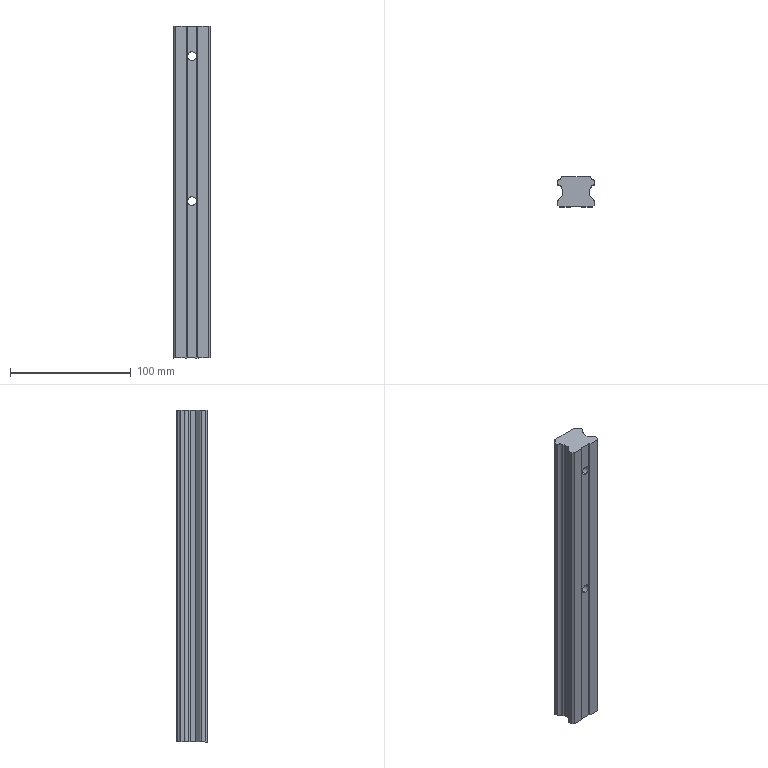Part | SolidWorks | features BaseBody 1 | 1 solid | 47 faces | box 30 x 25 x 275 mm | volume 176371 mm3 | cylinder 25 | plane 22 | commonest cylinder face diameters 1.2 x10 6 x5 7.2 x4 13 x4 2 x2